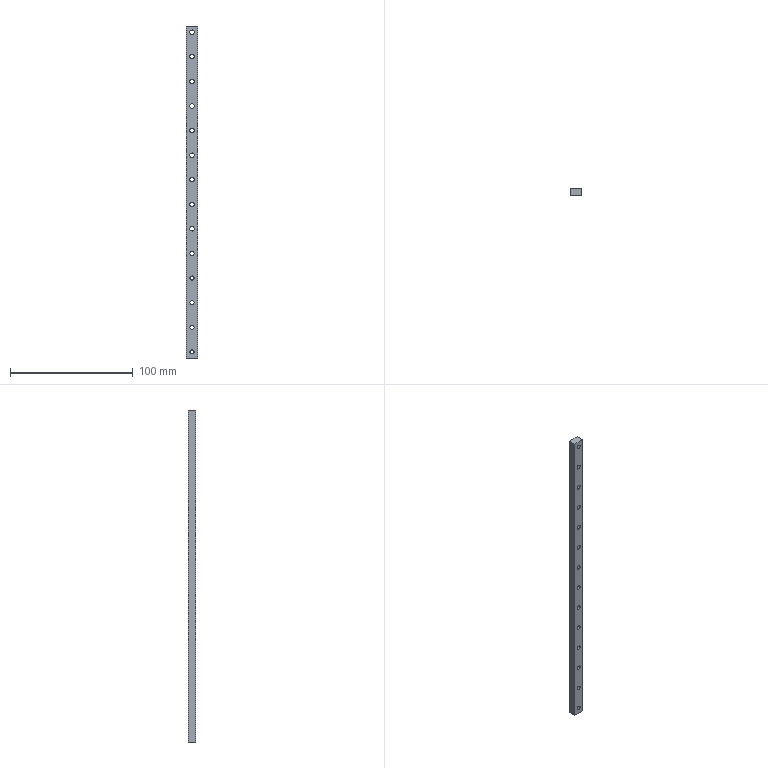Part | NX | features BREP 1 | 1 solid | 76 faces | box 9 x 6 x 270 mm | volume 12874 mm3 | cylinder 56 | plane 20 | commonest cylinder face diameters 6 x28 3.5 x18 3.4 x10